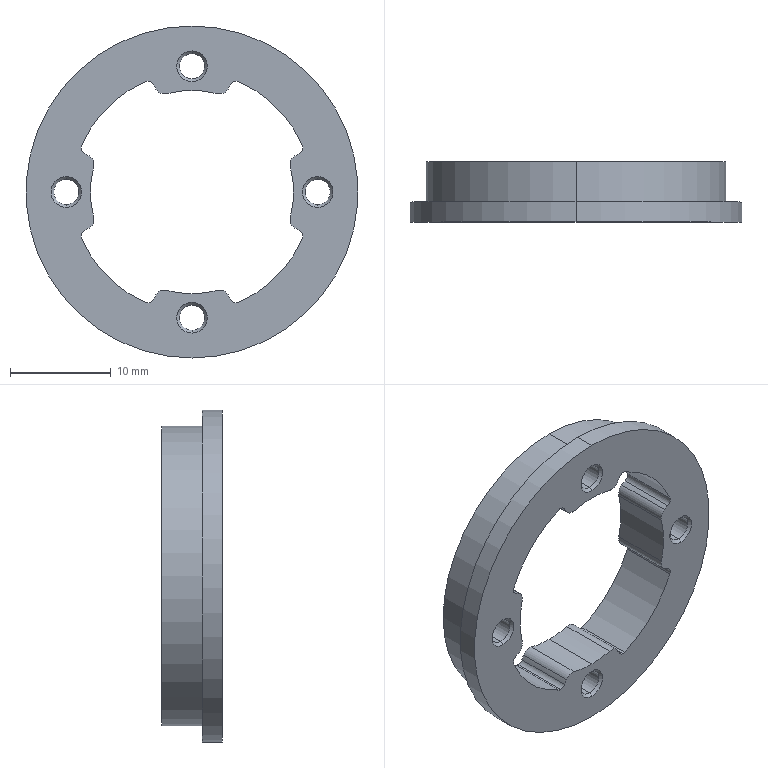Part | SolidWorks | features Fillet 2, Extrusion 1, HoleWzd 1, ICE 1, Shell 1 | 1 solid | 60 faces | box 33 x 6 x 33 mm | volume 2032 mm3 | cylinder 49 | cone 8 | plane 3 | commonest cylinder face diameters 1.2 x10 2 x10 2.5 x8 8.5 x8 20.2 x5 23.8 x4